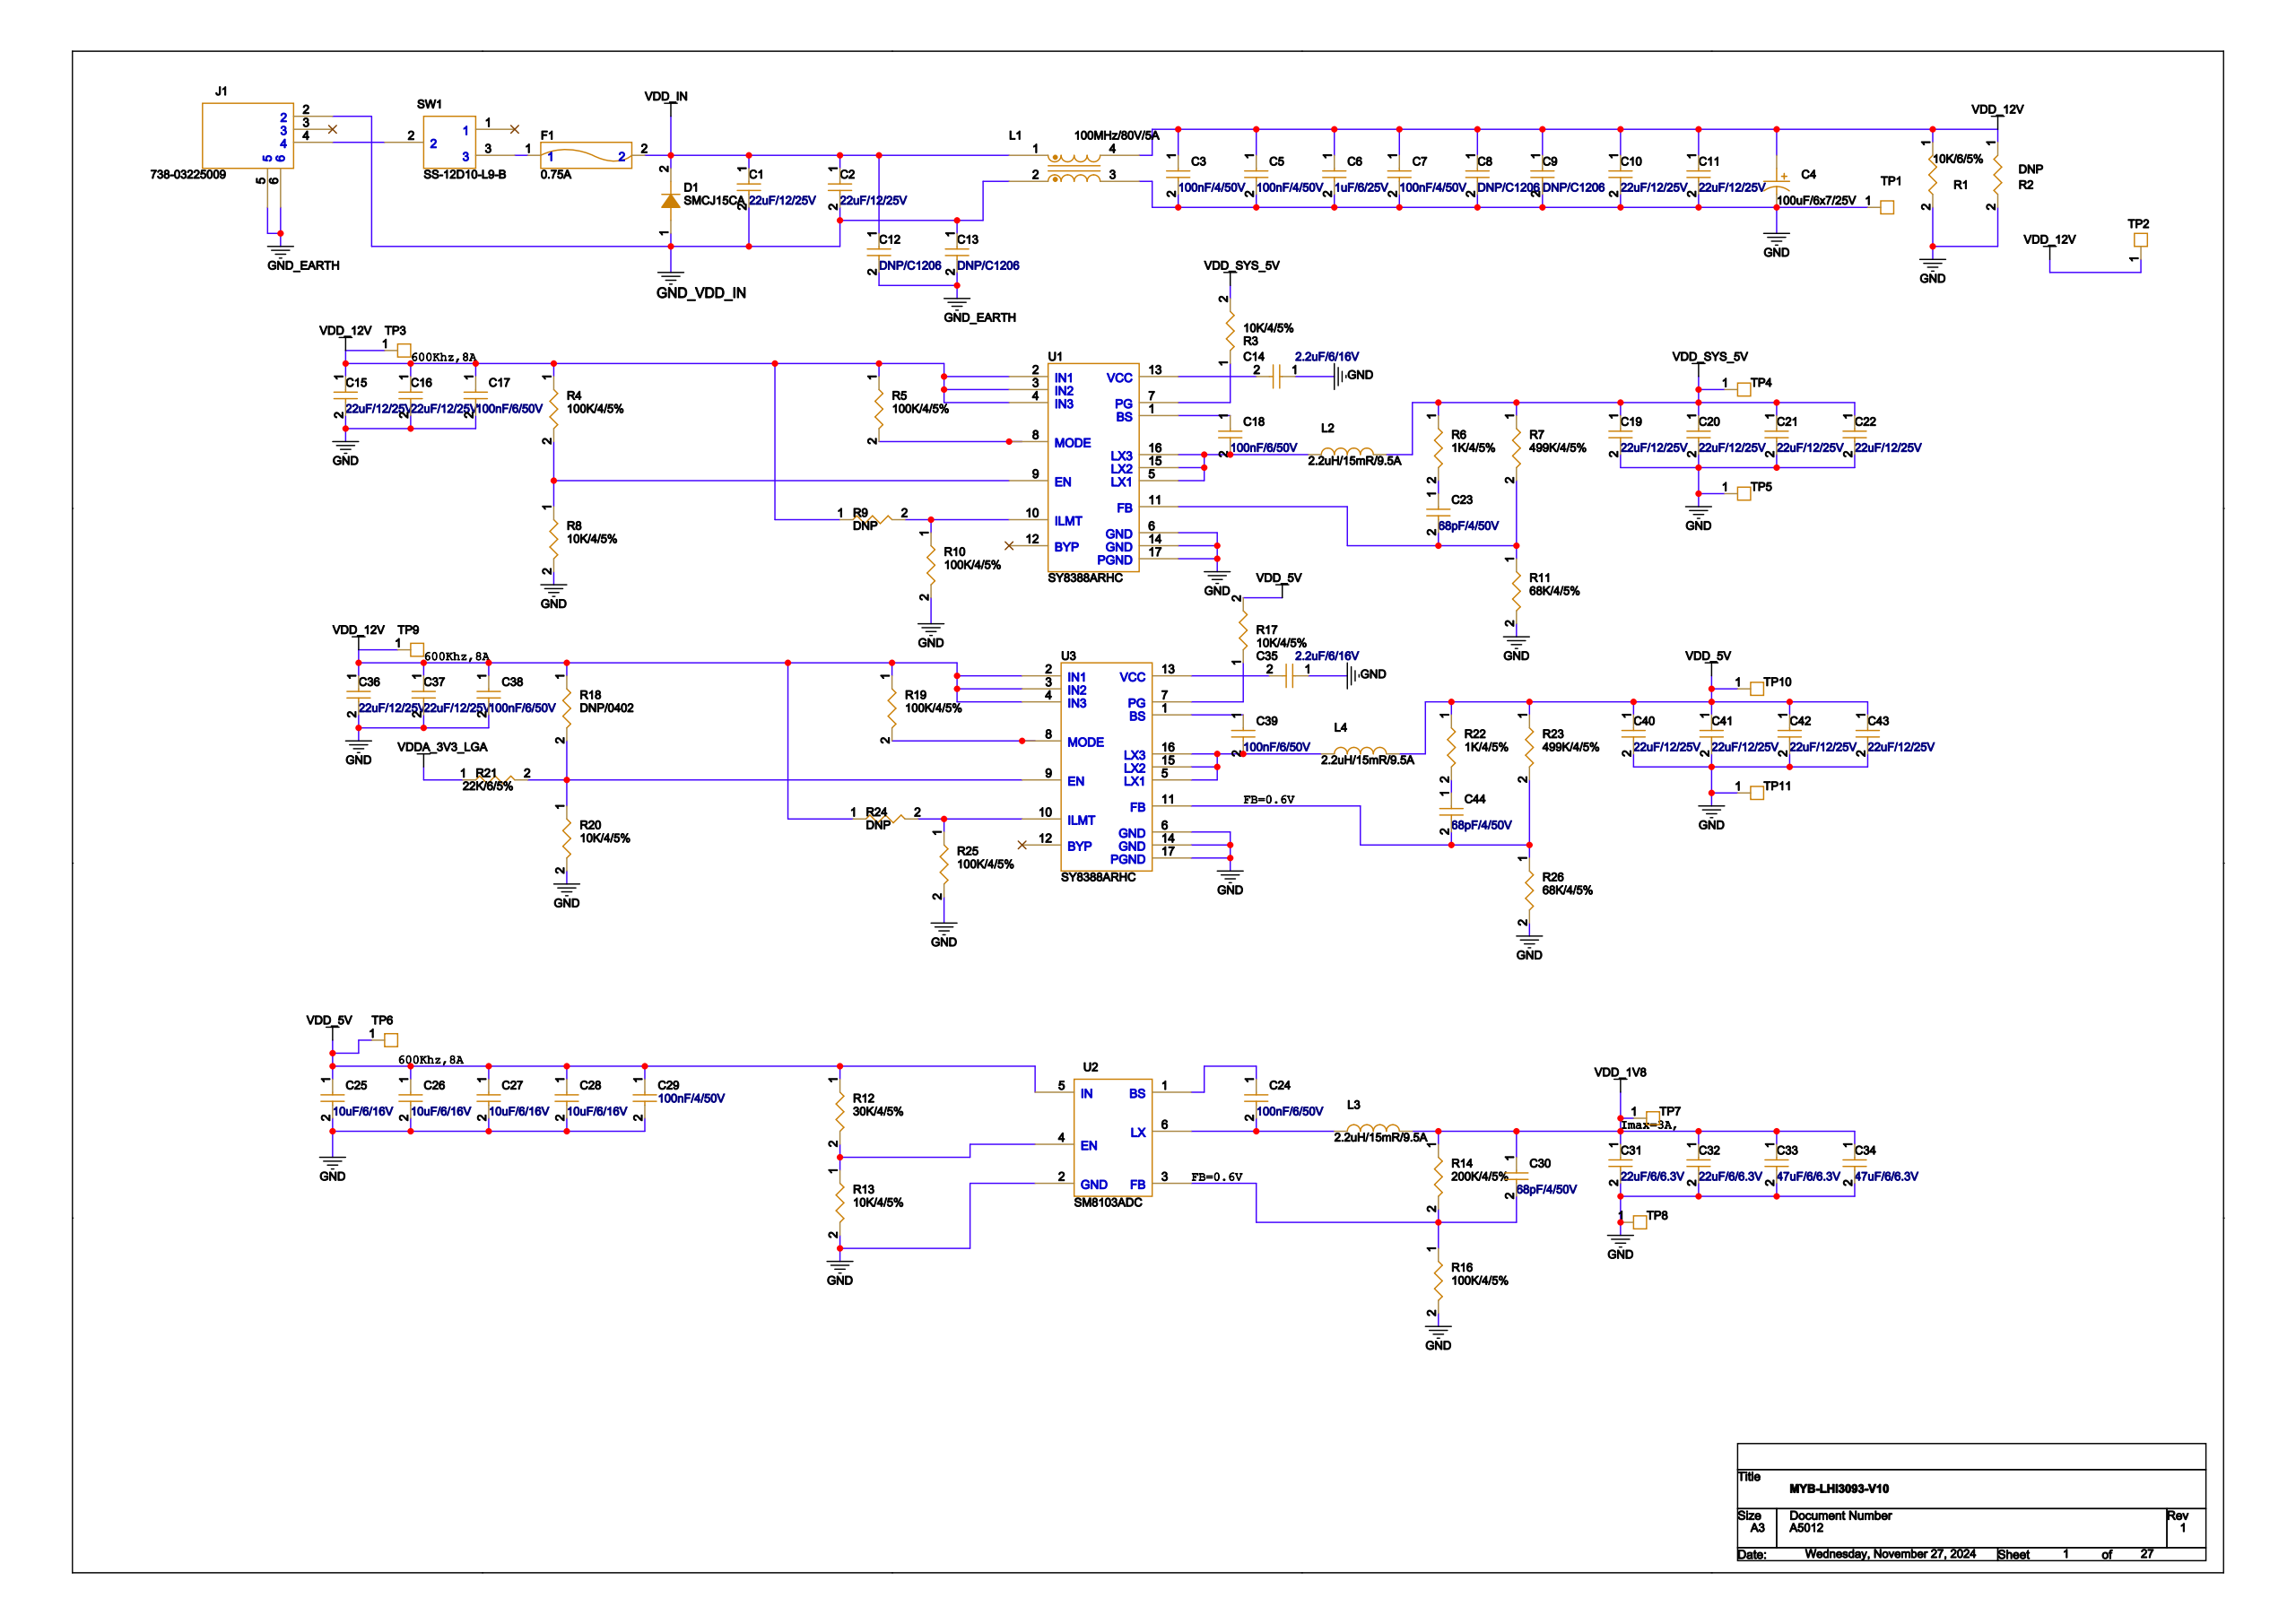Circuit board | Cadence Allegro | 1159 parts | 708 nets | one sheet of the schematic
Parts on this sheet (reference | value | footprint):
C1 | 22uF/12/25V | C1206
C2 | 22uF/12/25V | C1206
C3 | 100nF/4/50V | C0402
C4 | 100uF/6x7/25V | CE6X6
C5 | 100nF/4/50V | C0402
C6 | 1uF/6/25V | C0603
C7 | 100nF/4/50V | C0402
C8 | DNP/C1206 | C1206
C9 | DNP/C1206 | C1206
C10 | 22uF/12/25V | C1206
C11 | 22uF/12/25V | C1206
C12 | DNP/C1206 | C1206
C13 | DNP/C1206 | C1206
C14 | 2.2uF/6/16V | C0603
C15 | 22uF/12/25V | C1206
C16 | 22uF/12/25V | C1206
C17 | 100nF/6/50V | C0603
C18 | 100nF/6/50V | C0603
C19 | 22uF/12/25V | C1206
C20 | 22uF/12/25V | C1206
C21 | 22uF/12/25V | C1206
C22 | 22uF/12/25V | C1206
C23 | 68pF/4/50V | C0402
C24 | 100nF/6/50V | C0603
C25 | 10uF/6/16V | C0603
C26 | 10uF/6/16V | C0603
C27 | 10uF/6/16V | C0603
C28 | 10uF/6/16V | C0603
C29 | 100nF/4/50V | C0402
C30 | 68pF/4/50V | C0402
C31 | 22uF/6/6.3V | C0603
C32 | 22uF/6/6.3V | C0603
C33 | 47uF/6/6.3V | C0603
C34 | 47uF/6/6.3V | C0603
C35 | 2.2uF/6/16V | C0603
C36 | 22uF/12/25V | C1206
C37 | 22uF/12/25V | C1206
C38 | 100nF/6/50V | C0603
C39 | 100nF/6/50V | C0603
C40 | 22uF/12/25V | C1206
C41 | 22uF/12/25V | C1206
C42 | 22uF/12/25V | C1206
C43 | 22uF/12/25V | C1206
C44 | 68pF/4/50V | C0402
D1 | SMCJ15CA | DO-214AB
F1 | 0.75A | F1206
J1 | 738-03225009 | 738-032XX009
L1 | 100MHz/80V/5A | INDCM-ACM7060
L2 | 2.2uH/15mR/9.5A | L7X6_6
L3 | 2.2uH/15mR/9.5A | L4_85X4_7
L4 | 2.2uH/15mR/9.5A | L7X6_6
R1 | 10K/6/5% | R0603
R2 | DNP | R0402
R3 | 10K/4/5% | R0402
R4 | 100K/4/5% | R0402
R5 | 100K/4/5% | R0402
R6 | 1K/4/5% | R0402
R7 | 499K/4/5% | R0402
R8 | 10K/4/5% | R0402
R9 | DNP | R0402
R10 | 100K/4/5% | R0402
R11 | 68K/4/5% | R0402
R12 | 30K/4/5% | R0402
R13 | 10K/4/5% | R0402
R14 | 200K/4/5% | R0402
R16 | 100K/4/5% | R0402
R17 | 10K/4/5% | R0402
R18 | DNP/0402 | R0402
R19 | 100K/4/5% | R0402
R20 | 10K/4/5% | R0402
R21 | 22K/6/5% | R0603
R22 | 1K/4/5% | R0402
R23 | 499K/4/5% | R0402
R24 | DNP | R0402
R25 | 100K/4/5% | R0402
R26 | 68K/4/5% | R0402
SW1 | SS-12D10-L9-B | SW-SS-12D10-L9-B
TP1 | T POINT S | HOLE-TP0_9S16
TP2 | T POINT S | HOLE-TP0_9S16
TP3 | T POINT S | TPAD_020
TP4 | T POINT S | TPAD_020
TP5 | T POINT S | TPAD_020
TP6 | T POINT S | TPAD_020
TP7 | T POINT S | TPAD_020
TP8 | T POINT S | TPAD_020
TP9 | T POINT S | TPAD_020
TP10 | T POINT S | TPAD_020
TP11 | T POINT S | TPAD_020
U1 | SY8388ARHC | QFN16_0_45
U2 | SM8103ADC | SOT23-6
U3 | SY8388ARHC | QFN16_0_45
Nets of these parts (net: part-pin ...):
GND: C3-2 C4-2 C5-2 C6-2 C7-2 C8-2 C9-2 C10-2 C11-2 C14-1 C15-2 C16-2 C17-2 C19-2 C20-2 C21-2 C22-2 C25-2 C26-2 C27-2 C28-2 C29-2 C31-2 C32-2 C33-2 C34-2 C35-1 C36-2 C37-2 C38-2 C40-2 C41-2 C42-2 C43-2 L1-3 R1-2 R2-2 R8-2 R10-2 R11-2 R13-2 R16-2 R20-2 R25-2 R26-2 TP1-1 TP5-1 TP8-1 TP11-1 U1-6 U1-14 U1-17 U2-2 U3-6 U3-14 U3-17
VDD_IN: C1-1 C2-1 C12-1 D1-2 F1-2 L1-1
GND_VDD_IN: C1-2 C2-2 C13-1 D1-1 J1-2 L1-2
VDD_12V: C3-1 C4-1 C5-1 C6-1 C7-1 C8-1 C9-1 C10-1 C11-1 C15-1 C16-1 C17-1 C36-1 C37-1 C38-1 L1-4 R1-1 R2-1 R4-1 R5-1 R9-1 R18-1 R19-1 R24-1 TP2-1 TP3-1 TP9-1 U1-2 U1-3 U1-4 U3-2 U3-3 U3-4
VDD_SYS_5V: C19-1 C20-1 C21-1 C22-1 L2-2 R3-2 R6-1 R7-1 TP4-1
VDD_5V: C25-1 C26-1 C27-1 C28-1 C29-1 C40-1 C41-1 C42-1 C43-1 L4-2 R12-1 R17-2 R22-1 R23-1 TP6-1 TP10-1 U2-5
VDD_1V8: C30-1 C31-1 C32-1 C33-1 C34-1 L3-2 R14-1 TP7-1
GND_EARTH: C12-2 C13-2 J1-5 J1-6
N14897655: C14-2 U1-13
N14901269: C35-2 U3-13
N14897955: C18-1 U1-1
N14897959: C18-2 L2-1 U1-5 U1-15 U1-16
N14916956: C24-1 U2-1
N14916974: C24-2 L3-1 U2-6
N14901329: C39-1 U3-1
N14901333: C39-2 L4-1 U3-5 U3-15 U3-16
N14898208: C23-1 R6-2
N14898102: C23-2 R7-2 R11-1 U1-11
N14917095: C30-2 R14-2 R16-1 U2-3
N14901439: C44-1 R22-2
N14901381: C44-2 R23-2 R26-1 U3-11
N14891658: J1-4 SW1-2
N14896586: R9-2 R10-1 U1-10
N14901117: R19-2 U3-8
N14901153: R24-2 R25-1 U3-10
N14895732: R4-2 R8-1 U1-9
N14896357: R5-2 U1-8
N14916374: R12-2 R13-1 U2-4
N14901261: R17-1 U3-7
N14901045: R18-2 R20-1 R21-2 U3-9
N14897557: R3-1 U1-7
VDDA_3V3_LGA: R21-1
N14891817: F1-1 SW1-3